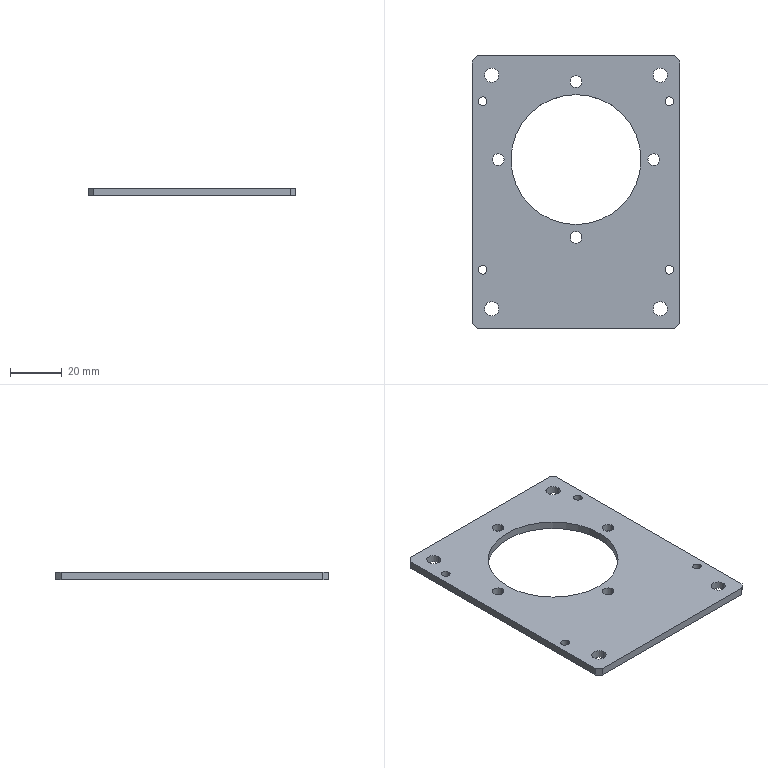Part | SolidWorks | features HoleWzd 2, Chamfer 1, Extrusion 1, ICE 1 | 1 solid | 36 faces | box 80 x 105 x 3 mm | volume 18683 mm3 | cylinder 26 | plane 10 | commonest cylinder face diameters 3.3 x8 4.5 x8 5.5 x8 50.1 x2
STEP:
#1=CARTESIAN_POINT('',(5.65,87.5,0.));
#2=VERTEX_POINT('',#1);
#3=CARTESIAN_POINT('',(2.35,87.5,0.));
#4=VERTEX_POINT('',#3);
#5=CARTESIAN_POINT('',(4.,87.5,0.));
#6=DIRECTION('',(0.,0.,-1.));
#7=DIRECTION('',(-1.,0.,0.));
#8=AXIS2_PLACEMENT_3D('',#5,#6,#7);
#9=CIRCLE('',#8,1.65);
#10=EDGE_CURVE('',#2,#4,#9,.T.);
#11=ORIENTED_EDGE('',*,*,#10,.T.);
#12=CARTESIAN_POINT('',(2.35,87.5,3.));
#13=VERTEX_POINT('',#12);
#14=CARTESIAN_POINT('',(2.35,87.5,3.));
#15=DIRECTION('',(0.,0.,1.));
#16=VECTOR('',#15,1000.);
#17=LINE('',#14,#16);
#18=EDGE_CURVE('',#4,#13,#17,.T.);
#19=ORIENTED_EDGE('',*,*,#18,.T.);
#20=CARTESIAN_POINT('',(5.65,87.5,3.));
#21=VERTEX_POINT('',#20);
#22=CARTESIAN_POINT('',(4.,87.5,3.));
#23=DIRECTION('',(0.,0.,1.));
#24=DIRECTION('',(1.,0.,0.));
#25=AXIS2_PLACEMENT_3D('',#22,#23,#24);
#26=CIRCLE('',#25,1.65);
#27=EDGE_CURVE('',#13,#21,#26,.T.);
#28=ORIENTED_EDGE('',*,*,#27,.T.);
#29=CARTESIAN_POINT('',(5.65,87.5,3.));
#30=DIRECTION('',(0.,0.,1.));
#31=VECTOR('',#30,1000.);
#32=LINE('',#29,#31);
#33=EDGE_CURVE('',#2,#21,#32,.T.);
#34=ORIENTED_EDGE('',*,*,#33,.F.);
#35=EDGE_LOOP('',(#11,#19,#28,#34));
#36=FACE_OUTER_BOUND('',#35,.T.);
#37=CARTESIAN_POINT('',(4.,87.5,3.));
#38=DIRECTION('',(0.,0.,1.));
#39=DIRECTION('',(1.,0.,0.));
#40=AXIS2_PLACEMENT_3D('',#37,#38,#39);
#41=CYLINDRICAL_SURFACE('',#40,1.65);
#42=ADVANCED_FACE('',(#36),#41,.F.);
#43=CARTESIAN_POINT('',(77.65,87.5,0.));
#44=VERTEX_POINT('',#43);
#45=CARTESIAN_POINT('',(74.35,87.5,0.));
#46=VERTEX_POINT('',#45);
#47=CARTESIAN_POINT('',(76.,87.5,0.));
#48=DIRECTION('',(0.,0.,-1.));
#49=DIRECTION('',(-1.,0.,0.));
#50=AXIS2_PLACEMENT_3D('',#47,#48,#49);
#51=CIRCLE('',#50,1.65);
#52=EDGE_CURVE('',#44,#46,#51,.T.);
#53=ORIENTED_EDGE('',*,*,#52,.T.);
#54=CARTESIAN_POINT('',(74.35,87.5,3.));
#55=VERTEX_POINT('',#54);
#56=CARTESIAN_POINT('',(74.35,87.5,3.));
#57=DIRECTION('',(0.,0.,1.));
#58=VECTOR('',#57,1000.);
#59=LINE('',#56,#58);
#60=EDGE_CURVE('',#46,#55,#59,.T.);
#61=ORIENTED_EDGE('',*,*,#60,.T.);
#62=CARTESIAN_POINT('',(77.65,87.5,3.));
#63=VERTEX_POINT('',#62);
#64=CARTESIAN_POINT('',(76.,87.5,3.));
#65=DIRECTION('',(0.,0.,1.));
#66=DIRECTION('',(1.,0.,0.));
#67=AXIS2_PLACEMENT_3D('',#64,#65,#66);
#68=CIRCLE('',#67,1.65);
#69=EDGE_CURVE('',#55,#63,#68,.T.);
#70=ORIENTED_EDGE('',*,*,#69,.T.);
#71=CARTESIAN_POINT('',(77.65,87.5,3.));
#72=DIRECTION('',(0.,0.,1.));
#73=VECTOR('',#72,1000.);
#74=LINE('',#71,#73);
#75=EDGE_CURVE('',#44,#63,#74,.T.);
#76=ORIENTED_EDGE('',*,*,#75,.F.);
#77=EDGE_LOOP('',(#53,#61,#70,#76));
#78=FACE_OUTER_BOUND('',#77,.T.);
#79=CARTESIAN_POINT('',(76.,87.5,3.));
#80=DIRECTION('',(0.,0.,1.));
#81=DIRECTION('',(1.,0.,0.));
#82=AXIS2_PLACEMENT_3D('',#79,#80,#81);
#83=CYLINDRICAL_SURFACE('',#82,1.65);
#84=ADVANCED_FACE('',(#78),#83,.F.);
#85=CARTESIAN_POINT('',(77.65,22.5,0.));
#86=VERTEX_POINT('',#85);
#87=CARTESIAN_POINT('',(74.35,22.5,0.));
#88=VERTEX_POINT('',#87);
#89=CARTESIAN_POINT('',(76.,22.5,0.));
#90=DIRECTION('',(0.,0.,-1.));
#91=DIRECTION('',(-1.,0.,0.));
#92=AXIS2_PLACEMENT_3D('',#89,#90,#91);
#93=CIRCLE('',#92,1.65);
#94=EDGE_CURVE('',#86,#88,#93,.T.);
#95=ORIENTED_EDGE('',*,*,#94,.T.);
#96=CARTESIAN_POINT('',(74.35,22.5,3.));
#97=VERTEX_POINT('',#96);
#98=CARTESIAN_POINT('',(74.35,22.5,3.));
#99=DIRECTION('',(0.,0.,1.));
#100=VECTOR('',#99,1000.);
#101=LINE('',#98,#100);
#102=EDGE_CURVE('',#88,#97,#101,.T.);
#103=ORIENTED_EDGE('',*,*,#102,.T.);
#104=CARTESIAN_POINT('',(77.65,22.5,3.));
#105=VERTEX_POINT('',#104);
#106=CARTESIAN_POINT('',(76.,22.5,3.));
#107=DIRECTION('',(0.,0.,1.));
#108=DIRECTION('',(1.,0.,0.));
#109=AXIS2_PLACEMENT_3D('',#106,#107,#108);
#110=CIRCLE('',#109,1.65);
#111=EDGE_CURVE('',#97,#105,#110,.T.);
#112=ORIENTED_EDGE('',*,*,#111,.T.);
#113=CARTESIAN_POINT('',(77.65,22.5,3.));
#114=DIRECTION('',(0.,0.,1.));
#115=VECTOR('',#114,1000.);
#116=LINE('',#113,#115);
#117=EDGE_CURVE('',#86,#105,#116,.T.);
#118=ORIENTED_EDGE('',*,*,#117,.F.);
#119=EDGE_LOOP('',(#95,#103,#112,#118));
#120=FACE_OUTER_BOUND('',#119,.T.);
#121=CARTESIAN_POINT('',(76.,22.5,3.));
#122=DIRECTION('',(0.,0.,1.));
#123=DIRECTION('',(1.,0.,0.));
#124=AXIS2_PLACEMENT_3D('',#121,#122,#123);
#125=CYLINDRICAL_SURFACE('',#124,1.65);
#126=ADVANCED_FACE('',(#120),#125,.F.);
#127=CARTESIAN_POINT('',(5.65,22.5,0.));
#128=VERTEX_POINT('',#127);
#129=CARTESIAN_POINT('',(2.35,22.5,0.));
#130=VERTEX_POINT('',#129);
#131=CARTESIAN_POINT('',(4.,22.5,0.));
#132=DIRECTION('',(0.,0.,-1.));
#133=DIRECTION('',(-1.,0.,0.));
#134=AXIS2_PLACEMENT_3D('',#131,#132,#133);
#135=CIRCLE('',#134,1.65);
#136=EDGE_CURVE('',#128,#130,#135,.T.);
#137=ORIENTED_EDGE('',*,*,#136,.T.);
#138=CARTESIAN_POINT('',(2.35,22.5,3.));
#139=VERTEX_POINT('',#138);
#140=CARTESIAN_POINT('',(2.35,22.5,3.));
#141=DIRECTION('',(0.,0.,1.));
#142=VECTOR('',#141,1000.);
#143=LINE('',#140,#142);
#144=EDGE_CURVE('',#130,#139,#143,.T.);
#145=ORIENTED_EDGE('',*,*,#144,.T.);
#146=CARTESIAN_POINT('',(5.65,22.5,3.));
#147=VERTEX_POINT('',#146);
#148=CARTESIAN_POINT('',(4.,22.5,3.));
#149=DIRECTION('',(0.,0.,1.));
#150=DIRECTION('',(1.,0.,0.));
#151=AXIS2_PLACEMENT_3D('',#148,#149,#150);
#152=CIRCLE('',#151,1.65);
#153=EDGE_CURVE('',#139,#147,#152,.T.);
#154=ORIENTED_EDGE('',*,*,#153,.T.);
#155=CARTESIAN_POINT('',(5.65,22.5,3.));
#156=DIRECTION('',(0.,0.,1.));
#157=VECTOR('',#156,1000.);
#158=LINE('',#155,#157);
#159=EDGE_CURVE('',#128,#147,#158,.T.);
#160=ORIENTED_EDGE('',*,*,#159,.F.);
#161=EDGE_LOOP('',(#137,#145,#154,#160));
#162=FACE_OUTER_BOUND('',#161,.T.);
#163=CARTESIAN_POINT('',(4.,22.5,3.));
#164=DIRECTION('',(0.,0.,1.));
#165=DIRECTION('',(1.,0.,0.));
#166=AXIS2_PLACEMENT_3D('',#163,#164,#165);
#167=CYLINDRICAL_SURFACE('',#166,1.65);
#168=ADVANCED_FACE('',(#162),#167,.F.);
#169=CARTESIAN_POINT('',(37.75,95.,0.));
#170=VERTEX_POINT('',#169);
#171=CARTESIAN_POINT('',(42.25,95.,0.));
#172=VERTEX_POINT('',#171);
#173=CARTESIAN_POINT('',(40.,95.,0.));
#174=DIRECTION('',(0.,0.,1.));
#175=DIRECTION('',(1.,0.,0.));
#176=AXIS2_PLACEMENT_3D('',#173,#174,#175);
#177=CIRCLE('',#176,2.25);
#178=EDGE_CURVE('',#170,#172,#177,.T.);
#179=ORIENTED_EDGE('',*,*,#178,.F.);
#180=CARTESIAN_POINT('',(37.75,95.,3.));
#181=VERTEX_POINT('',#180);
#182=CARTESIAN_POINT('',(37.75,95.,3.));
#183=DIRECTION('',(0.,0.,1.));
#184=VECTOR('',#183,1000.);
#185=LINE('',#182,#184);
#186=EDGE_CURVE('',#170,#181,#185,.T.);
#187=ORIENTED_EDGE('',*,*,#186,.T.);
#188=CARTESIAN_POINT('',(42.25,95.,3.));
#189=VERTEX_POINT('',#188);
#190=CARTESIAN_POINT('',(40.,95.,3.));
#191=DIRECTION('',(0.,0.,1.));
#192=DIRECTION('',(1.,0.,0.));
#193=AXIS2_PLACEMENT_3D('',#190,#191,#192);
#194=CIRCLE('',#193,2.25);
#195=EDGE_CURVE('',#181,#189,#194,.T.);
#196=ORIENTED_EDGE('',*,*,#195,.T.);
#197=CARTESIAN_POINT('',(42.25,95.,3.));
#198=DIRECTION('',(0.,0.,1.));
#199=VECTOR('',#198,1000.);
#200=LINE('',#197,#199);
#201=EDGE_CURVE('',#172,#189,#200,.T.);
#202=ORIENTED_EDGE('',*,*,#201,.F.);
#203=EDGE_LOOP('',(#179,#187,#196,#202));
#204=FACE_OUTER_BOUND('',#203,.T.);
#205=CARTESIAN_POINT('',(40.,95.,3.));
#206=DIRECTION('',(0.,0.,1.));
#207=DIRECTION('',(1.,0.,0.));
#208=AXIS2_PLACEMENT_3D('',#205,#206,#207);
#209=CYLINDRICAL_SURFACE('',#208,2.25);
#210=ADVANCED_FACE('',(#204),#209,.F.);
#211=CARTESIAN_POINT('',(7.75,65.,0.));
#212=VERTEX_POINT('',#211);
#213=CARTESIAN_POINT('',(12.25,65.,0.));
#214=VERTEX_POINT('',#213);
#215=CARTESIAN_POINT('',(10.,65.,0.));
#216=DIRECTION('',(0.,0.,1.));
#217=DIRECTION('',(1.,0.,0.));
#218=AXIS2_PLACEMENT_3D('',#215,#216,#217);
#219=CIRCLE('',#218,2.25);
#220=EDGE_CURVE('',#212,#214,#219,.T.);
#221=ORIENTED_EDGE('',*,*,#220,.F.);
#222=CARTESIAN_POINT('',(7.75,65.,3.));
#223=VERTEX_POINT('',#222);
#224=CARTESIAN_POINT('',(7.75,65.,3.));
#225=DIRECTION('',(0.,0.,1.));
#226=VECTOR('',#225,1000.);
#227=LINE('',#224,#226);
#228=EDGE_CURVE('',#212,#223,#227,.T.);
#229=ORIENTED_EDGE('',*,*,#228,.T.);
#230=CARTESIAN_POINT('',(12.25,65.,3.));
#231=VERTEX_POINT('',#230);
#232=CARTESIAN_POINT('',(10.,65.,3.));
#233=DIRECTION('',(0.,0.,1.));
#234=DIRECTION('',(1.,0.,0.));
#235=AXIS2_PLACEMENT_3D('',#232,#233,#234);
#236=CIRCLE('',#235,2.25);
#237=EDGE_CURVE('',#223,#231,#236,.T.);
#238=ORIENTED_EDGE('',*,*,#237,.T.);
#239=CARTESIAN_POINT('',(12.25,65.,3.));
#240=DIRECTION('',(0.,0.,1.));
#241=VECTOR('',#240,1000.);
#242=LINE('',#239,#241);
#243=EDGE_CURVE('',#214,#231,#242,.T.);
#244=ORIENTED_EDGE('',*,*,#243,.F.);
#245=EDGE_LOOP('',(#221,#229,#238,#244));
#246=FACE_OUTER_BOUND('',#245,.T.);
#247=CARTESIAN_POINT('',(10.,65.,3.));
#248=DIRECTION('',(0.,0.,1.));
#249=DIRECTION('',(1.,0.,0.));
#250=AXIS2_PLACEMENT_3D('',#247,#248,#249);
#251=CYLINDRICAL_SURFACE('',#250,2.25);
#252=ADVANCED_FACE('',(#246),#251,.F.);
#253=CARTESIAN_POINT('',(67.75,65.,0.));
#254=VERTEX_POINT('',#253);
#255=CARTESIAN_POINT('',(72.25,65.,0.));
#256=VERTEX_POINT('',#255);
#257=CARTESIAN_POINT('',(70.,65.,0.));
#258=DIRECTION('',(0.,0.,1.));
#259=DIRECTION('',(1.,0.,0.));
#260=AXIS2_PLACEMENT_3D('',#257,#258,#259);
#261=CIRCLE('',#260,2.25);
#262=EDGE_CURVE('',#254,#256,#261,.T.);
#263=ORIENTED_EDGE('',*,*,#262,.F.);
#264=CARTESIAN_POINT('',(67.75,65.,3.));
#265=VERTEX_POINT('',#264);
#266=CARTESIAN_POINT('',(67.75,65.,3.));
#267=DIRECTION('',(0.,0.,1.));
#268=VECTOR('',#267,1000.);
#269=LINE('',#266,#268);
#270=EDGE_CURVE('',#254,#265,#269,.T.);
#271=ORIENTED_EDGE('',*,*,#270,.T.);
#272=CARTESIAN_POINT('',(72.25,65.,3.));
#273=VERTEX_POINT('',#272);
#274=CARTESIAN_POINT('',(70.,65.,3.));
#275=DIRECTION('',(0.,0.,1.));
#276=DIRECTION('',(1.,0.,0.));
#277=AXIS2_PLACEMENT_3D('',#274,#275,#276);
#278=CIRCLE('',#277,2.25);
#279=EDGE_CURVE('',#265,#273,#278,.T.);
#280=ORIENTED_EDGE('',*,*,#279,.T.);
#281=CARTESIAN_POINT('',(72.25,65.,3.));
#282=DIRECTION('',(0.,0.,1.));
#283=VECTOR('',#282,1000.);
#284=LINE('',#281,#283);
#285=EDGE_CURVE('',#256,#273,#284,.T.);
#286=ORIENTED_EDGE('',*,*,#285,.F.);
#287=EDGE_LOOP('',(#263,#271,#280,#286));
#288=FACE_OUTER_BOUND('',#287,.T.);
#289=CARTESIAN_POINT('',(70.,65.,3.));
#290=DIRECTION('',(0.,0.,1.));
#291=DIRECTION('',(1.,0.,0.));
#292=AXIS2_PLACEMENT_3D('',#289,#290,#291);
#293=CYLINDRICAL_SURFACE('',#292,2.25);
#294=ADVANCED_FACE('',(#288),#293,.F.);
#295=CARTESIAN_POINT('',(37.75,35.,0.));
#296=VERTEX_POINT('',#295);
#297=CARTESIAN_POINT('',(42.25,35.,0.));
#298=VERTEX_POINT('',#297);
#299=CARTESIAN_POINT('',(40.,35.,0.));
#300=DIRECTION('',(0.,0.,1.));
#301=DIRECTION('',(1.,0.,0.));
#302=AXIS2_PLACEMENT_3D('',#299,#300,#301);
#303=CIRCLE('',#302,2.25);
#304=EDGE_CURVE('',#296,#298,#303,.T.);
#305=ORIENTED_EDGE('',*,*,#304,.F.);
#306=CARTESIAN_POINT('',(37.75,35.,3.));
#307=VERTEX_POINT('',#306);
#308=CARTESIAN_POINT('',(37.75,35.,3.));
#309=DIRECTION('',(0.,0.,1.));
#310=VECTOR('',#309,1000.);
#311=LINE('',#308,#310);
#312=EDGE_CURVE('',#296,#307,#311,.T.);
#313=ORIENTED_EDGE('',*,*,#312,.T.);
#314=CARTESIAN_POINT('',(42.25,35.,3.));
#315=VERTEX_POINT('',#314);
#316=CARTESIAN_POINT('',(40.,35.,3.));
#317=DIRECTION('',(0.,0.,1.));
#318=DIRECTION('',(1.,0.,0.));
#319=AXIS2_PLACEMENT_3D('',#316,#317,#318);
#320=CIRCLE('',#319,2.25);
#321=EDGE_CURVE('',#307,#315,#320,.T.);
#322=ORIENTED_EDGE('',*,*,#321,.T.);
#323=CARTESIAN_POINT('',(42.25,35.,3.));
#324=DIRECTION('',(0.,0.,1.));
#325=VECTOR('',#324,1000.);
#326=LINE('',#323,#325);
#327=EDGE_CURVE('',#298,#315,#326,.T.);
#328=ORIENTED_EDGE('',*,*,#327,.F.);
#329=EDGE_LOOP('',(#305,#313,#322,#328));
#330=FACE_OUTER_BOUND('',#329,.T.);
#331=CARTESIAN_POINT('',(40.,35.,3.));
#332=DIRECTION('',(0.,0.,1.));
#333=DIRECTION('',(1.,0.,0.));
#334=AXIS2_PLACEMENT_3D('',#331,#332,#333);
#335=CYLINDRICAL_SURFACE('',#334,2.25);
#336=ADVANCED_FACE('',(#330),#335,.F.);
#337=CARTESIAN_POINT('',(14.95,65.,0.));
#338=VERTEX_POINT('',#337);
#339=CARTESIAN_POINT('',(65.05,65.,0.));
#340=VERTEX_POINT('',#339);
#341=CARTESIAN_POINT('',(40.,65.,0.));
#342=DIRECTION('',(0.,0.,1.));
#343=DIRECTION('',(1.,0.,0.));
#344=AXIS2_PLACEMENT_3D('',#341,#342,#343);
#345=CIRCLE('',#344,25.05);
#346=EDGE_CURVE('',#338,#340,#345,.T.);
#347=ORIENTED_EDGE('',*,*,#346,.F.);
#348=CARTESIAN_POINT('',(14.95,65.,3.));
#349=VERTEX_POINT('',#348);
#350=CARTESIAN_POINT('',(14.95,65.,0.));
#351=DIRECTION('',(0.,0.,1.));
#352=VECTOR('',#351,1000.);
#353=LINE('',#350,#352);
#354=EDGE_CURVE('',#338,#349,#353,.T.);
#355=ORIENTED_EDGE('',*,*,#354,.T.);
#356=CARTESIAN_POINT('',(65.05,65.,3.));
#357=VERTEX_POINT('',#356);
#358=CARTESIAN_POINT('',(40.,65.,3.));
#359=DIRECTION('',(0.,0.,1.));
#360=DIRECTION('',(1.,0.,0.));
#361=AXIS2_PLACEMENT_3D('',#358,#359,#360);
#362=CIRCLE('',#361,25.05);
#363=EDGE_CURVE('',#349,#357,#362,.T.);
#364=ORIENTED_EDGE('',*,*,#363,.T.);
#365=CARTESIAN_POINT('',(65.05,65.,0.));
#366=DIRECTION('',(0.,0.,1.));
#367=VECTOR('',#366,1000.);
#368=LINE('',#365,#367);
#369=EDGE_CURVE('',#340,#357,#368,.T.);
#370=ORIENTED_EDGE('',*,*,#369,.F.);
#371=EDGE_LOOP('',(#347,#355,#364,#370));
#372=FACE_OUTER_BOUND('',#371,.T.);
#373=CARTESIAN_POINT('',(40.,65.,0.));
#374=DIRECTION('',(0.,0.,1.));
#375=DIRECTION('',(1.,0.,0.));
#376=AXIS2_PLACEMENT_3D('',#373,#374,#375);
#377=CYLINDRICAL_SURFACE('',#376,25.05);
#378=ADVANCED_FACE('',(#372),#377,.F.);
#379=CARTESIAN_POINT('',(4.75,7.5,0.));
#380=VERTEX_POINT('',#379);
#381=CARTESIAN_POINT('',(10.25,7.5,0.));
#382=VERTEX_POINT('',#381);
#383=CARTESIAN_POINT('',(7.5,7.5,0.));
#384=DIRECTION('',(0.,0.,1.));
#385=DIRECTION('',(1.,0.,0.));
#386=AXIS2_PLACEMENT_3D('',#383,#384,#385);
#387=CIRCLE('',#386,2.75);
#388=EDGE_CURVE('',#380,#382,#387,.T.);
#389=ORIENTED_EDGE('',*,*,#388,.F.);
#390=CARTESIAN_POINT('',(4.75,7.5,3.));
#391=VERTEX_POINT('',#390);
#392=CARTESIAN_POINT('',(4.75,7.5,0.));
#393=DIRECTION('',(0.,0.,1.));
#394=VECTOR('',#393,1000.);
#395=LINE('',#392,#394);
#396=EDGE_CURVE('',#380,#391,#395,.T.);
#397=ORIENTED_EDGE('',*,*,#396,.T.);
#398=CARTESIAN_POINT('',(10.25,7.5,3.));
#399=VERTEX_POINT('',#398);
#400=CARTESIAN_POINT('',(7.5,7.5,3.));
#401=DIRECTION('',(0.,0.,1.));
#402=DIRECTION('',(1.,0.,0.));
#403=AXIS2_PLACEMENT_3D('',#400,#401,#402);
#404=CIRCLE('',#403,2.75);
#405=EDGE_CURVE('',#391,#399,#404,.T.);
#406=ORIENTED_EDGE('',*,*,#405,.T.);
#407=CARTESIAN_POINT('',(10.25,7.5,0.));
#408=DIRECTION('',(0.,0.,1.));
#409=VECTOR('',#408,1000.);
#410=LINE('',#407,#409);
#411=EDGE_CURVE('',#382,#399,#410,.T.);
#412=ORIENTED_EDGE('',*,*,#411,.F.);
#413=EDGE_LOOP('',(#389,#397,#406,#412));
#414=FACE_OUTER_BOUND('',#413,.T.);
#415=CARTESIAN_POINT('',(7.5,7.5,0.));
#416=DIRECTION('',(0.,0.,1.));
#417=DIRECTION('',(1.,0.,0.));
#418=AXIS2_PLACEMENT_3D('',#415,#416,#417);
#419=CYLINDRICAL_SURFACE('',#418,2.75);
#420=ADVANCED_FACE('',(#414),#419,.F.);
#421=CARTESIAN_POINT('',(69.75,7.5,0.));
#422=VERTEX_POINT('',#421);
#423=CARTESIAN_POINT('',(75.25,7.5,0.));
#424=VERTEX_POINT('',#423);
#425=CARTESIAN_POINT('',(72.5,7.5,0.));
#426=DIRECTION('',(0.,0.,1.));
#427=DIRECTION('',(1.,0.,0.));
#428=AXIS2_PLACEMENT_3D('',#425,#426,#427);
#429=CIRCLE('',#428,2.75);
#430=EDGE_CURVE('',#422,#424,#429,.T.);
#431=ORIENTED_EDGE('',*,*,#430,.F.);
#432=CARTESIAN_POINT('',(69.75,7.5,3.));
#433=VERTEX_POINT('',#432);
#434=CARTESIAN_POINT('',(69.75,7.5,0.));
#435=DIRECTION('',(0.,0.,1.));
#436=VECTOR('',#435,1000.);
#437=LINE('',#434,#436);
#438=EDGE_CURVE('',#422,#433,#437,.T.);
#439=ORIENTED_EDGE('',*,*,#438,.T.);
#440=CARTESIAN_POINT('',(75.25,7.5,3.));
#441=VERTEX_POINT('',#440);
#442=CARTESIAN_POINT('',(72.5,7.5,3.));
#443=DIRECTION('',(0.,0.,1.));
#444=DIRECTION('',(1.,0.,0.));
#445=AXIS2_PLACEMENT_3D('',#442,#443,#444);
#446=CIRCLE('',#445,2.75);
#447=EDGE_CURVE('',#433,#441,#446,.T.);
#448=ORIENTED_EDGE('',*,*,#447,.T.);
#449=CARTESIAN_POINT('',(75.25,7.5,0.));
#450=DIRECTION('',(0.,0.,1.));
#451=VECTOR('',#450,1000.);
#452=LINE('',#449,#451);
#453=EDGE_CURVE('',#424,#441,#452,.T.);
#454=ORIENTED_EDGE('',*,*,#453,.F.);
#455=EDGE_LOOP('',(#431,#439,#448,#454));
#456=FACE_OUTER_BOUND('',#455,.T.);
#457=CARTESIAN_POINT('',(72.5,7.5,0.));
#458=DIRECTION('',(0.,0.,1.));
#459=DIRECTION('',(1.,0.,0.));
#460=AXIS2_PLACEMENT_3D('',#457,#458,#459);
#461=CYLINDRICAL_SURFACE('',#460,2.75);
#462=ADVANCED_FACE('',(#456),#461,.F.);
#463=CARTESIAN_POINT('',(69.75,97.5,0.));
#464=VERTEX_POINT('',#463);
#465=CARTESIAN_POINT('',(75.25,97.5,0.));
#466=VERTEX_POINT('',#465);
#467=CARTESIAN_POINT('',(72.5,97.5,0.));
#468=DIRECTION('',(0.,0.,1.));
#469=DIRECTION('',(1.,0.,0.));
#470=AXIS2_PLACEMENT_3D('',#467,#468,#469);
#471=CIRCLE('',#470,2.75);
#472=EDGE_CURVE('',#464,#466,#471,.T.);
#473=ORIENTED_EDGE('',*,*,#472,.F.);
#474=CARTESIAN_POINT('',(69.75,97.5,3.));
#475=VERTEX_POINT('',#474);
#476=CARTESIAN_POINT('',(69.75,97.5,0.));
#477=DIRECTION('',(0.,0.,1.));
#478=VECTOR('',#477,1000.);
#479=LINE('',#476,#478);
#480=EDGE_CURVE('',#464,#475,#479,.T.);
#481=ORIENTED_EDGE('',*,*,#480,.T.);
#482=CARTESIAN_POINT('',(75.25,97.5,3.));
#483=VERTEX_POINT('',#482);
#484=CARTESIAN_POINT('',(72.5,97.5,3.));
#485=DIRECTION('',(0.,0.,1.));
#486=DIRECTION('',(1.,0.,0.));
#487=AXIS2_PLACEMENT_3D('',#484,#485,#486);
#488=CIRCLE('',#487,2.75);
#489=EDGE_CURVE('',#475,#483,#488,.T.);
#490=ORIENTED_EDGE('',*,*,#489,.T.);
#491=CARTESIAN_POINT('',(75.25,97.5,0.));
#492=DIRECTION('',(0.,0.,1.));
#493=VECTOR('',#492,1000.);
#494=LINE('',#491,#493);
#495=EDGE_CURVE('',#466,#483,#494,.T.);
#496=ORIENTED_EDGE('',*,*,#495,.F.);
#497=EDGE_LOOP('',(#473,#481,#490,#496));
#498=FACE_OUTER_BOUND('',#497,.T.);
#499=CARTESIAN_POINT('',(72.5,97.5,0.));
#500=DIRECTION('',(0.,0.,1.));
#501=DIRECTION('',(1.,0.,0.));
#502=AXIS2_PLACEMENT_3D('',#499,#500,#501);
#503=CYLINDRICAL_SURFACE('',#502,2.75);
#504=ADVANCED_FACE('',(#498),#503,.F.);
#505=CARTESIAN_POINT('',(4.75,97.5,0.));
#506=VERTEX_POINT('',#505);
#507=CARTESIAN_POINT('',(10.25,97.5,0.));
#508=VERTEX_POINT('',#507);
#509=CARTESIAN_POINT('',(7.5,97.5,0.));
#510=DIRECTION('',(0.,0.,1.));
#511=DIRECTION('',(1.,0.,0.));
#512=AXIS2_PLACEMENT_3D('',#509,#510,#511);
#513=CIRCLE('',#512,2.75);
#514=EDGE_CURVE('',#506,#508,#513,.T.);
#515=ORIENTED_EDGE('',*,*,#514,.F.);
#516=CARTESIAN_POINT('',(4.75,97.5,3.));
#517=VERTEX_POINT('',#516);
#518=CARTESIAN_POINT('',(4.75,97.5,0.));
#519=DIRECTION('',(0.,0.,1.));
#520=VECTOR('',#519,1000.);
#521=LINE('',#518,#520);
#522=EDGE_CURVE('',#506,#517,#521,.T.);
#523=ORIENTED_EDGE('',*,*,#522,.T.);
#524=CARTESIAN_POINT('',(10.25,97.5,3.));
#525=VERTEX_POINT('',#524);
#526=CARTESIAN_POINT('',(7.5,97.5,3.));
#527=DIRECTION('',(0.,0.,1.));
#528=DIRECTION('',(1.,0.,0.));
#529=AXIS2_PLACEMENT_3D('',#526,#527,#528);
#530=CIRCLE('',#529,2.75);
#531=EDGE_CURVE('',#517,#525,#530,.T.);
#532=ORIENTED_EDGE('',*,*,#531,.T.);
#533=CARTESIAN_POINT('',(10.25,97.5,0.));
#534=DIRECTION('',(0.,0.,1.));
#535=VECTOR('',#534,1000.);
#536=LINE('',#533,#535);
#537=EDGE_CURVE('',#508,#525,#536,.T.);
#538=ORIENTED_EDGE('',*,*,#537,.F.);
#539=EDGE_LOOP('',(#515,#523,#532,#538));
#540=FACE_OUTER_BOUND('',#539,.T.);
#541=CARTESIAN_POINT('',(7.5,97.5,0.));
#542=DIRECTION('',(0.,0.,1.));
#543=DIRECTION('',(1.,0.,0.));
#544=AXIS2_PLACEMENT_3D('',#541,#542,#543);
#545=CYLINDRICAL_SURFACE('',#544,2.75);
#546=ADVANCED_FACE('',(#540),#545,.F.);
#547=CARTESIAN_POINT('',(0.,103.,0.));
#548=VERTEX_POINT('',#547);
#549=CARTESIAN_POINT('',(0.,2.,0.));
#550=VERTEX_POINT('',#549);
#551=CARTESIAN_POINT('',(0.,0.,0.));
#552=DIRECTION('',(0.,-1.,0.));
#553=VECTOR('',#552,1000.);
#554=LINE('',#551,#553);
#555=EDGE_CURVE('',#548,#550,#554,.T.);
#556=ORIENTED_EDGE('',*,*,#555,.T.);
#557=CARTESIAN_POINT('',(0.,2.,3.));
#558=VERTEX_POINT('',#557);
#559=CARTESIAN_POINT('',(0.,2.,3.));
#560=DIRECTION('',(0.,0.,1.));
#561=VECTOR('',#560,1000.);
#562=LINE('',#559,#561);
#563=EDGE_CURVE('',#550,#558,#562,.T.);
#564=ORIENTED_EDGE('',*,*,#563,.T.);
#565=CARTESIAN_POINT('',(0.,103.,3.));
#566=VERTEX_POINT('',#565);
#567=CARTESIAN_POINT('',(0.,0.,3.));
#568=DIRECTION('',(0.,-1.,0.));
#569=VECTOR('',#568,1000.);
#570=LINE('',#567,#569);
#571=EDGE_CURVE('',#566,#558,#570,.T.);
#572=ORIENTED_EDGE('',*,*,#571,.F.);
#573=CARTESIAN_POINT('',(0.,103.,3.));
#574=DIRECTION('',(0.,0.,-1.));
#575=VECTOR('',#574,1000.);
#576=LINE('',#573,#575);
#577=EDGE_CURVE('',#566,#548,#576,.T.);
#578=ORIENTED_EDGE('',*,*,#577,.T.);
#579=EDGE_LOOP('',(#556,#564,#572,#578));
#580=FACE_OUTER_BOUND('',#579,.T.);
#581=CARTESIAN_POINT('',(0.,0.,3.));
#582=DIRECTION('',(1.,0.,0.));
#583=DIRECTION('',(0.,0.,-1.));
#584=AXIS2_PLACEMENT_3D('',#581,#582,#583);
#585=PLANE('',#584);
#586=ADVANCED_FACE('',(#580),#585,.F.);
#587=CARTESIAN_POINT('',(2.,0.,0.));
#588=VERTEX_POINT('',#587);
#589=CARTESIAN_POINT('',(78.,0.,0.));
#590=VERTEX_POINT('',#589);
#591=CARTESIAN_POINT('',(0.,0.,0.));
#592=DIRECTION('',(1.,0.,0.));
#593=VECTOR('',#592,1000.);
#594=LINE('',#591,#593);
#595=EDGE_CURVE('',#588,#590,#594,.T.);
#596=ORIENTED_EDGE('',*,*,#595,.T.);
#597=CARTESIAN_POINT('',(78.,0.,3.));
#598=VERTEX_POINT('',#597);
#599=CARTESIAN_POINT('',(78.,0.,3.));
#600=DIRECTION('',(0.,0.,1.));
#601=VECTOR('',#600,1000.);
#602=LINE('',#599,#601);
#603=EDGE_CURVE('',#590,#598,#602,.T.);
#604=ORIENTED_EDGE('',*,*,#603,.T.);
#605=CARTESIAN_POINT('',(2.,0.,3.));
#606=VERTEX_POINT('',#605);
#607=CARTESIAN_POINT('',(0.,0.,3.));
#608=DIRECTION('',(1.,0.,0.));
#609=VECTOR('',#608,1000.);
#610=LINE('',#607,#609);
#611=EDGE_CURVE('',#606,#598,#610,.T.);
#612=ORIENTED_EDGE('',*,*,#611,.F.);
#613=CARTESIAN_POINT('',(2.,0.,3.));
#614=DIRECTION('',(0.,0.,-1.));
#615=VECTOR('',#614,1000.);
#616=LINE('',#613,#615);
#617=EDGE_CURVE('',#606,#588,#616,.T.);
#618=ORIENTED_EDGE('',*,*,#617,.T.);
#619=EDGE_LOOP('',(#596,#604,#612,#618));
#620=FACE_OUTER_BOUND('',#619,.T.);
#621=CARTESIAN_POINT('',(0.,0.,3.));
#622=DIRECTION('',(0.,1.,0.));
#623=DIRECTION('',(0.,0.,1.));
#624=AXIS2_PLACEMENT_3D('',#621,#622,#623);
#625=PLANE('',#624);
#626=ADVANCED_FACE('',(#620),#625,.F.);
#627=CARTESIAN_POINT('',(80.,2.,3.));
#628=VERTEX_POINT('',#627);
#629=CARTESIAN_POINT('',(80.,103.,3.));
#630=VERTEX_POINT('',#629);
#631=CARTESIAN_POINT('',(80.,0.,3.));
#632=DIRECTION('',(0.,1.,0.));
#633=VECTOR('',#632,1000.);
#634=LINE('',#631,#633);
#635=EDGE_CURVE('',#628,#630,#634,.T.);
#636=ORIENTED_EDGE('',*,*,#635,.F.);
#637=CARTESIAN_POINT('',(80.,2.,0.));
#638=VERTEX_POINT('',#637);
#639=CARTESIAN_POINT('',(80.,2.,3.));
#640=DIRECTION('',(0.,0.,-1.));
#641=VECTOR('',#640,1000.);
#642=LINE('',#639,#641);
#643=EDGE_CURVE('',#628,#638,#642,.T.);
#644=ORIENTED_EDGE('',*,*,#643,.T.);
#645=CARTESIAN_POINT('',(80.,103.,0.));
#646=VERTEX_POINT('',#645);
#647=CARTESIAN_POINT('',(80.,0.,0.));
#648=DIRECTION('',(0.,1.,0.));
#649=VECTOR('',#648,1000.);
#650=LINE('',#647,#649);
#651=EDGE_CURVE('',#638,#646,#650,.T.);
#652=ORIENTED_EDGE('',*,*,#651,.T.);
#653=CARTESIAN_POINT('',(80.,103.,3.));
#654=DIRECTION('',(0.,0.,1.));
#655=VECTOR('',#654,1000.);
#656=LINE('',#653,#655);
#657=EDGE_CURVE('',#646,#630,#656,.T.);
#658=ORIENTED_EDGE('',*,*,#657,.T.);
#659=EDGE_LOOP('',(#636,#644,#652,#658));
#660=FACE_OUTER_BOUND('',#659,.T.);
#661=CARTESIAN_POINT('',(80.,0.,3.));
#662=DIRECTION('',(-1.,0.,0.));
#663=DIRECTION('',(0.,0.,1.));
#664=AXIS2_PLACEMENT_3D('',#661,#662,#663);
#665=PLANE('',#664);
#666=ADVANCED_FACE('',(#660),#665,.F.);
#667=CARTESIAN_POINT('',(78.,105.,3.));
#668=VERTEX_POINT('',#667);
#669=CARTESIAN_POINT('',(2.,105.,3.));
#670=VERTEX_POINT('',#669);
#671=CARTESIAN_POINT('',(0.,105.,3.));
#672=DIRECTION('',(-1.,0.,0.));
#673=VECTOR('',#672,1000.);
#674=LINE('',#671,#673);
#675=EDGE_CURVE('',#668,#670,#674,.T.);
#676=ORIENTED_EDGE('',*,*,#675,.F.);
#677=CARTESIAN_POINT('',(78.,105.,0.));
#678=VERTEX_POINT('',#677);
#679=CARTESIAN_POINT('',(78.,105.,3.));
#680=DIRECTION('',(0.,0.,-1.));
#681=VECTOR('',#680,1000.);
#682=LINE('',#679,#681);
#683=EDGE_CURVE('',#668,#678,#682,.T.);
#684=ORIENTED_EDGE('',*,*,#683,.T.);
#685=CARTESIAN_POINT('',(2.,105.,0.));
#686=VERTEX_POINT('',#685);
#687=CARTESIAN_POINT('',(0.,105.,0.));
#688=DIRECTION('',(-1.,0.,0.));
#689=VECTOR('',#688,1000.);
#690=LINE('',#687,#689);
#691=EDGE_CURVE('',#678,#686,#690,.T.);
#692=ORIENTED_EDGE('',*,*,#691,.T.);
#693=CARTESIAN_POINT('',(2.,105.,3.));
#694=DIRECTION('',(0.,0.,1.));
#695=VECTOR('',#694,1000.);
#696=LINE('',#693,#695);
#697=EDGE_CURVE('',#686,#670,#696,.T.);
#698=ORIENTED_EDGE('',*,*,#697,.T.);
#699=EDGE_LOOP('',(#676,#684,#692,#698));
#700=FACE_OUTER_BOUND('',#699,.T.);
#701=CARTESIAN_POINT('',(0.,105.,3.));
#702=DIRECTION('',(0.,-1.,0.));
#703=DIRECTION('',(0.,0.,-1.));
#704=AXIS2_PLACEMENT_3D('',#701,#702,#703);
#705=PLANE('',#704);
#706=ADVANCED_FACE('',(#700),#705,.F.);
#707=CARTESIAN_POINT('',(4.,87.5,3.));
#708=DIRECTION('',(0.,0.,1.));
#709=DIRECTION('',(1.,0.,0.));
#710=AXIS2_PLACEMENT_3D('',#707,#708,#709);
#711=CIRCLE('',#710,1.65);
#712=EDGE_CURVE('',#21,#13,#711,.T.);
#713=ORIENTED_EDGE('',*,*,#712,.F.);
#714=ORIENTED_EDGE('',*,*,#27,.F.);
#715=EDGE_LOOP('',(#713,#714));
#716=FACE_BOUND('',#715,.T.);
#717=CARTESIAN_POINT('',(76.,87.5,3.));
#718=DIRECTION('',(0.,0.,1.));
#719=DIRECTION('',(1.,0.,0.));
#720=AXIS2_PLACEMENT_3D('',#717,#718,#719);
#721=CIRCLE('',#720,1.65);
#722=EDGE_CURVE('',#63,#55,#721,.T.);
#723=ORIENTED_EDGE('',*,*,#722,.F.);
#724=ORIENTED_EDGE('',*,*,#69,.F.);
#725=EDGE_LOOP('',(#723,#724));
#726=FACE_BOUND('',#725,.T.);
#727=CARTESIAN_POINT('',(76.,22.5,3.));
#728=DIRECTION('',(0.,0.,1.));
#729=DIRECTION('',(1.,0.,0.));
#730=AXIS2_PLACEMENT_3D('',#727,#728,#729);
#731=CIRCLE('',#730,1.65);
#732=EDGE_CURVE('',#105,#97,#731,.T.);
#733=ORIENTED_EDGE('',*,*,#732,.F.);
#734=ORIENTED_EDGE('',*,*,#111,.F.);
#735=EDGE_LOOP('',(#733,#734));
#736=FACE_BOUND('',#735,.T.);
#737=CARTESIAN_POINT('',(4.,22.5,3.));
#738=DIRECTION('',(0.,0.,1.));
#739=DIRECTION('',(1.,0.,0.));
#740=AXIS2_PLACEMENT_3D('',#737,#738,#739);
#741=CIRCLE('',#740,1.65);
#742=EDGE_CURVE('',#147,#139,#741,.T.);
#743=ORIENTED_EDGE('',*,*,#742,.F.);
#744=ORIENTED_EDGE('',*,*,#153,.F.);
#745=EDGE_LOOP('',(#743,#744));
#746=FACE_BOUND('',#745,.T.);
#747=CARTESIAN_POINT('',(40.,95.,3.));
#748=DIRECTION('',(0.,0.,1.));
#749=DIRECTION('',(1.,0.,0.));
#750=AXIS2_PLACEMENT_3D('',#747,#748,#749);
#751=CIRCLE('',#750,2.25);
#752=EDGE_CURVE('',#189,#181,#751,.T.);
#753=ORIENTED_EDGE('',*,*,#752,.F.);
#754=ORIENTED_EDGE('',*,*,#195,.F.);
#755=EDGE_LOOP('',(#753,#754));
#756=FACE_BOUND('',#755,.T.);
#757=CARTESIAN_POINT('',(10.,65.,3.));
#758=DIRECTION('',(0.,0.,1.));
#759=DIRECTION('',(1.,0.,0.));
#760=AXIS2_PLACEMENT_3D('',#757,#758,#759);
#761=CIRCLE('',#760,2.25);
#762=EDGE_CURVE('',#231,#223,#761,.T.);
#763=ORIENTED_EDGE('',*,*,#762,.F.);
#764=ORIENTED_EDGE('',*,*,#237,.F.);
#765=EDGE_LOOP('',(#763,#764));
#766=FACE_BOUND('',#765,.T.);
#767=CARTESIAN_POINT('',(70.,65.,3.));
#768=DIRECTION('',(0.,0.,1.));
#769=DIRECTION('',(1.,0.,0.));
#770=AXIS2_PLACEMENT_3D('',#767,#768,#769);
#771=CIRCLE('',#770,2.25);
#772=EDGE_CURVE('',#273,#265,#771,.T.);
#773=ORIENTED_EDGE('',*,*,#772,.F.);
#774=ORIENTED_EDGE('',*,*,#279,.F.);
#775=EDGE_LOOP('',(#773,#774));
#776=FACE_BOUND('',#775,.T.);
#777=CARTESIAN_POINT('',(40.,35.,3.));
#778=DIRECTION('',(0.,0.,1.));
#779=DIRECTION('',(1.,0.,0.));
#780=AXIS2_PLACEMENT_3D('',#777,#778,#779);
#781=CIRCLE('',#780,2.25);
#782=EDGE_CURVE('',#315,#307,#781,.T.);
#783=ORIENTED_EDGE('',*,*,#782,.F.);
#784=ORIENTED_EDGE('',*,*,#321,.F.);
#785=EDGE_LOOP('',(#783,#784));
#786=FACE_BOUND('',#785,.T.);
#787=CARTESIAN_POINT('',(40.,65.,3.));
#788=DIRECTION('',(0.,0.,1.));
#789=DIRECTION('',(1.,0.,0.));
#790=AXIS2_PLACEMENT_3D('',#787,#788,#789);
#791=CIRCLE('',#790,25.05);
#792=EDGE_CURVE('',#357,#349,#791,.T.);
#793=ORIENTED_EDGE('',*,*,#792,.F.);
#794=ORIENTED_EDGE('',*,*,#363,.F.);
#795=EDGE_LOOP('',(#793,#794));
#796=FACE_BOUND('',#795,.T.);
#797=CARTESIAN_POINT('',(7.5,7.5,3.));
#798=DIRECTION('',(0.,0.,1.));
#799=DIRECTION('',(1.,0.,0.));
#800=AXIS2_PLACEMENT_3D('',#797,#798,#799);
#801=CIRCLE('',#800,2.75);
#802=EDGE_CURVE('',#399,#391,#801,.T.);
#803=ORIENTED_EDGE('',*,*,#802,.F.);
#804=ORIENTED_EDGE('',*,*,#405,.F.);
#805=EDGE_LOOP('',(#803,#804));
#806=FACE_BOUND('',#805,.T.);
#807=CARTESIAN_POINT('',(72.5,7.5,3.));
#808=DIRECTION('',(0.,0.,1.));
#809=DIRECTION('',(1.,0.,0.));
#810=AXIS2_PLACEMENT_3D('',#807,#808,#809);
#811=CIRCLE('',#810,2.75);
#812=EDGE_CURVE('',#441,#433,#811,.T.);
#813=ORIENTED_EDGE('',*,*,#812,.F.);
#814=ORIENTED_EDGE('',*,*,#447,.F.);
#815=EDGE_LOOP('',(#813,#814));
#816=FACE_BOUND('',#815,.T.);
#817=CARTESIAN_POINT('',(72.5,97.5,3.));
#818=DIRECTION('',(0.,0.,1.));
#819=DIRECTION('',(1.,0.,0.));
#820=AXIS2_PLACEMENT_3D('',#817,#818,#819);
#821=CIRCLE('',#820,2.75);
#822=EDGE_CURVE('',#483,#475,#821,.T.);
#823=ORIENTED_EDGE('',*,*,#822,.F.);
#824=ORIENTED_EDGE('',*,*,#489,.F.);
#825=EDGE_LOOP('',(#823,#824));
#826=FACE_BOUND('',#825,.T.);
#827=CARTESIAN_POINT('',(7.5,97.5,3.));
#828=DIRECTION('',(0.,0.,1.));
#829=DIRECTION('',(1.,0.,0.));
#830=AXIS2_PLACEMENT_3D('',#827,#828,#829);
#831=CIRCLE('',#830,2.75);
#832=EDGE_CURVE('',#525,#517,#831,.T.);
#833=ORIENTED_EDGE('',*,*,#832,.F.);
#834=ORIENTED_EDGE('',*,*,#531,.F.);
#835=EDGE_LOOP('',(#833,#834));
#836=FACE_BOUND('',#835,.T.);
#837=ORIENTED_EDGE('',*,*,#611,.T.);
#838=CARTESIAN_POINT('',(80.,2.,3.));
#839=DIRECTION('',(0.7071,0.7071,0.));
#840=VECTOR('',#839,1000.);
#841=LINE('',#838,#840);
#842=EDGE_CURVE('',#598,#628,#841,.T.);
#843=ORIENTED_EDGE('',*,*,#842,.T.);
#844=ORIENTED_EDGE('',*,*,#635,.T.);
#845=CARTESIAN_POINT('',(78.,105.,3.));
#846=DIRECTION('',(-0.7071,0.7071,0.));
#847=VECTOR('',#846,1000.);
#848=LINE('',#845,#847);
#849=EDGE_CURVE('',#630,#668,#848,.T.);
#850=ORIENTED_EDGE('',*,*,#849,.T.);
#851=ORIENTED_EDGE('',*,*,#675,.T.);
#852=CARTESIAN_POINT('',(0.,103.,3.));
#853=DIRECTION('',(-0.7071,-0.7071,0.));
#854=VECTOR('',#853,1000.);
#855=LINE('',#852,#854);
#856=EDGE_CURVE('',#670,#566,#855,.T.);
#857=ORIENTED_EDGE('',*,*,#856,.T.);
#858=ORIENTED_EDGE('',*,*,#571,.T.);
#859=CARTESIAN_POINT('',(2.,0.,3.));
#860=DIRECTION('',(0.7071,-0.7071,0.));
#861=VECTOR('',#860,1000.);
#862=LINE('',#859,#861);
#863=EDGE_CURVE('',#558,#606,#862,.T.);
#864=ORIENTED_EDGE('',*,*,#863,.T.);
#865=EDGE_LOOP('',(#837,#843,#844,#850,#851,#857,#858,#864));
#866=FACE_OUTER_BOUND('',#865,.T.);
#867=CARTESIAN_POINT('',(0.,105.,3.));
#868=DIRECTION('',(0.,0.,-1.));
#869=DIRECTION('',(-1.,0.,0.));
#870=AXIS2_PLACEMENT_3D('',#867,#868,#869);
#871=PLANE('',#870);
#872=ADVANCED_FACE('',(#716,#726,#736,#746,#756,#766,#776,#786,#796,#806,#816,#826,#836,#866),#871,.F.);
#873=ORIENTED_EDGE('',*,*,#10,.F.);
#874=CARTESIAN_POINT('',(4.,87.5,0.));
#875=DIRECTION('',(0.,0.,-1.));
#876=DIRECTION('',(-1.,0.,0.));
#877=AXIS2_PLACEMENT_3D('',#874,#875,#876);
#878=CIRCLE('',#877,1.65);
#879=EDGE_CURVE('',#4,#2,#878,.T.);
#880=ORIENTED_EDGE('',*,*,#879,.F.);
#881=EDGE_LOOP('',(#873,#880));
#882=FACE_BOUND('',#881,.T.);
#883=ORIENTED_EDGE('',*,*,#52,.F.);
#884=CARTESIAN_POINT('',(76.,87.5,0.));
#885=DIRECTION('',(0.,0.,-1.));
#886=DIRECTION('',(-1.,0.,0.));
#887=AXIS2_PLACEMENT_3D('',#884,#885,#886);
#888=CIRCLE('',#887,1.65);
#889=EDGE_CURVE('',#46,#44,#888,.T.);
#890=ORIENTED_EDGE('',*,*,#889,.F.);
#891=EDGE_LOOP('',(#883,#890));
#892=FACE_BOUND('',#891,.T.);
#893=ORIENTED_EDGE('',*,*,#94,.F.);
#894=CARTESIAN_POINT('',(76.,22.5,0.));
#895=DIRECTION('',(0.,0.,-1.));
#896=DIRECTION('',(-1.,0.,0.));
#897=AXIS2_PLACEMENT_3D('',#894,#895,#896);
#898=CIRCLE('',#897,1.65);
#899=EDGE_CURVE('',#88,#86,#898,.T.);
#900=ORIENTED_EDGE('',*,*,#899,.F.);
#901=EDGE_LOOP('',(#893,#900));
#902=FACE_BOUND('',#901,.T.);
#903=ORIENTED_EDGE('',*,*,#136,.F.);
#904=CARTESIAN_POINT('',(4.,22.5,0.));
#905=DIRECTION('',(0.,0.,-1.));
#906=DIRECTION('',(-1.,0.,0.));
#907=AXIS2_PLACEMENT_3D('',#904,#905,#906);
#908=CIRCLE('',#907,1.65);
#909=EDGE_CURVE('',#130,#128,#908,.T.);
#910=ORIENTED_EDGE('',*,*,#909,.F.);
#911=EDGE_LOOP('',(#903,#910));
#912=FACE_BOUND('',#911,.T.);
#913=CARTESIAN_POINT('',(40.,95.,0.));
#914=DIRECTION('',(0.,0.,1.));
#915=DIRECTION('',(1.,0.,0.));
#916=AXIS2_PLACEMENT_3D('',#913,#914,#915);
#917=CIRCLE('',#916,2.25);
#918=EDGE_CURVE('',#172,#170,#917,.T.);
#919=ORIENTED_EDGE('',*,*,#918,.T.);
#920=ORIENTED_EDGE('',*,*,#178,.T.);
#921=EDGE_LOOP('',(#919,#920));
#922=FACE_BOUND('',#921,.T.);
#923=CARTESIAN_POINT('',(10.,65.,0.));
#924=DIRECTION('',(0.,0.,1.));
#925=DIRECTION('',(1.,0.,0.));
#926=AXIS2_PLACEMENT_3D('',#923,#924,#925);
#927=CIRCLE('',#926,2.25);
#928=EDGE_CURVE('',#214,#212,#927,.T.);
#929=ORIENTED_EDGE('',*,*,#928,.T.);
#930=ORIENTED_EDGE('',*,*,#220,.T.);
#931=EDGE_LOOP('',(#929,#930));
#932=FACE_BOUND('',#931,.T.);
#933=CARTESIAN_POINT('',(70.,65.,0.));
#934=DIRECTION('',(0.,0.,1.));
#935=DIRECTION('',(1.,0.,0.));
#936=AXIS2_PLACEMENT_3D('',#933,#934,#935);
#937=CIRCLE('',#936,2.25);
#938=EDGE_CURVE('',#256,#254,#937,.T.);
#939=ORIENTED_EDGE('',*,*,#938,.T.);
#940=ORIENTED_EDGE('',*,*,#262,.T.);
#941=EDGE_LOOP('',(#939,#940));
#942=FACE_BOUND('',#941,.T.);
#943=CARTESIAN_POINT('',(40.,35.,0.));
#944=DIRECTION('',(0.,0.,1.));
#945=DIRECTION('',(1.,0.,0.));
#946=AXIS2_PLACEMENT_3D('',#943,#944,#945);
#947=CIRCLE('',#946,2.25);
#948=EDGE_CURVE('',#298,#296,#947,.T.);
#949=ORIENTED_EDGE('',*,*,#948,.T.);
#950=ORIENTED_EDGE('',*,*,#304,.T.);
#951=EDGE_LOOP('',(#949,#950));
#952=FACE_BOUND('',#951,.T.);
#953=CARTESIAN_POINT('',(40.,65.,0.));
#954=DIRECTION('',(0.,0.,1.));
#955=DIRECTION('',(1.,0.,0.));
#956=AXIS2_PLACEMENT_3D('',#953,#954,#955);
#957=CIRCLE('',#956,25.05);
#958=EDGE_CURVE('',#340,#338,#957,.T.);
#959=ORIENTED_EDGE('',*,*,#958,.T.);
#960=ORIENTED_EDGE('',*,*,#346,.T.);
#961=EDGE_LOOP('',(#959,#960));
#962=FACE_BOUND('',#961,.T.);
#963=CARTESIAN_POINT('',(7.5,7.5,0.));
#964=DIRECTION('',(0.,0.,1.));
#965=DIRECTION('',(1.,0.,0.));
#966=AXIS2_PLACEMENT_3D('',#963,#964,#965);
#967=CIRCLE('',#966,2.75);
#968=EDGE_CURVE('',#382,#380,#967,.T.);
#969=ORIENTED_EDGE('',*,*,#968,.T.);
#970=ORIENTED_EDGE('',*,*,#388,.T.);
#971=EDGE_LOOP('',(#969,#970));
#972=FACE_BOUND('',#971,.T.);
#973=CARTESIAN_POINT('',(72.5,7.5,0.));
#974=DIRECTION('',(0.,0.,1.));
#975=DIRECTION('',(1.,0.,0.));
#976=AXIS2_PLACEMENT_3D('',#973,#974,#975);
#977=CIRCLE('',#976,2.75);
#978=EDGE_CURVE('',#424,#422,#977,.T.);
#979=ORIENTED_EDGE('',*,*,#978,.T.);
#980=ORIENTED_EDGE('',*,*,#430,.T.);
#981=EDGE_LOOP('',(#979,#980));
#982=FACE_BOUND('',#981,.T.);
#983=CARTESIAN_POINT('',(72.5,97.5,0.));
#984=DIRECTION('',(0.,0.,1.));
#985=DIRECTION('',(1.,0.,0.));
#986=AXIS2_PLACEMENT_3D('',#983,#984,#985);
#987=CIRCLE('',#986,2.75);
#988=EDGE_CURVE('',#466,#464,#987,.T.);
#989=ORIENTED_EDGE('',*,*,#988,.T.);
#990=ORIENTED_EDGE('',*,*,#472,.T.);
#991=EDGE_LOOP('',(#989,#990));
#992=FACE_BOUND('',#991,.T.);
#993=CARTESIAN_POINT('',(7.5,97.5,0.));
#994=DIRECTION('',(0.,0.,1.));
#995=DIRECTION('',(1.,0.,0.));
#996=AXIS2_PLACEMENT_3D('',#993,#994,#995);
#997=CIRCLE('',#996,2.75);
#998=EDGE_CURVE('',#508,#506,#997,.T.);
#999=ORIENTED_EDGE('',*,*,#998,.T.);
#1000=ORIENTED_EDGE('',*,*,#514,.T.);
#1001=EDGE_LOOP('',(#999,#1000));
#1002=FACE_BOUND('',#1001,.T.);
#1003=ORIENTED_EDGE('',*,*,#651,.F.);
#1004=CARTESIAN_POINT('',(91.5,13.5,0.));
#1005=DIRECTION('',(-0.7071,-0.7071,0.));
#1006=VECTOR('',#1005,1000.);
#1007=LINE('',#1004,#1006);
#1008=EDGE_CURVE('',#638,#590,#1007,.T.);
#1009=ORIENTED_EDGE('',*,*,#1008,.T.);
#1010=ORIENTED_EDGE('',*,*,#595,.F.);
#1011=CARTESIAN_POINT('',(-51.5,53.5,0.));
#1012=DIRECTION('',(-0.7071,0.7071,0.));
#1013=VECTOR('',#1012,1000.);
#1014=LINE('',#1011,#1013);
#1015=EDGE_CURVE('',#588,#550,#1014,.T.);
#1016=ORIENTED_EDGE('',*,*,#1015,.T.);
#1017=ORIENTED_EDGE('',*,*,#555,.F.);
#1018=CARTESIAN_POINT('',(1.,104.,0.));
#1019=DIRECTION('',(0.7071,0.7071,0.));
#1020=VECTOR('',#1019,1000.);
#1021=LINE('',#1018,#1020);
#1022=EDGE_CURVE('',#548,#686,#1021,.T.);
#1023=ORIENTED_EDGE('',*,*,#1022,.T.);
#1024=ORIENTED_EDGE('',*,*,#691,.F.);
#1025=CARTESIAN_POINT('',(39.,144.,0.));
#1026=DIRECTION('',(0.7071,-0.7071,0.));
#1027=VECTOR('',#1026,1000.);
#1028=LINE('',#1025,#1027);
#1029=EDGE_CURVE('',#678,#646,#1028,.T.);
#1030=ORIENTED_EDGE('',*,*,#1029,.T.);
#1031=EDGE_LOOP('',(#1003,#1009,#1010,#1016,#1017,#1023,#1024,#1030));
#1032=FACE_OUTER_BOUND('',#1031,.T.);
#1033=CARTESIAN_POINT('',(0.,105.,0.));
#1034=DIRECTION('',(0.,0.,-1.));
#1035=DIRECTION('',(-1.,0.,0.));
#1036=AXIS2_PLACEMENT_3D('',#1033,#1034,#1035);
#1037=PLANE('',#1036);
#1038=ADVANCED_FACE('',(#882,#892,#902,#912,#922,#932,#942,#952,#962,#972,#982,#992,#1002,#1032),#1037,.T.);
#1039=ORIENTED_EDGE('',*,*,#522,.F.);
#1040=ORIENTED_EDGE('',*,*,#998,.F.);
#1041=ORIENTED_EDGE('',*,*,#537,.T.);
#1042=ORIENTED_EDGE('',*,*,#832,.T.);
#1043=EDGE_LOOP('',(#1039,#1040,#1041,#1042));
#1044=FACE_OUTER_BOUND('',#1043,.T.);
#1045=CARTESIAN_POINT('',(7.5,97.5,0.));
#1046=DIRECTION('',(0.,0.,1.));
#1047=DIRECTION('',(1.,0.,0.));
#1048=AXIS2_PLACEMENT_3D('',#1045,#1046,#1047);
#1049=CYLINDRICAL_SURFACE('',#1048,2.75);
#1050=ADVANCED_FACE('',(#1044),#1049,.F.);
#1051=ORIENTED_EDGE('',*,*,#480,.F.);
#1052=ORIENTED_EDGE('',*,*,#988,.F.);
#1053=ORIENTED_EDGE('',*,*,#495,.T.);
#1054=ORIENTED_EDGE('',*,*,#822,.T.);
#1055=EDGE_LOOP('',(#1051,#1052,#1053,#1054));
#1056=FACE_OUTER_BOUND('',#1055,.T.);
#1057=CARTESIAN_POINT('',(72.5,97.5,0.));
#1058=DIRECTION('',(0.,0.,1.));
#1059=DIRECTION('',(1.,0.,0.));
#1060=AXIS2_PLACEMENT_3D('',#1057,#1058,#1059);
#1061=CYLINDRICAL_SURFACE('',#1060,2.75);
#1062=ADVANCED_FACE('',(#1056),#1061,.F.);
#1063=ORIENTED_EDGE('',*,*,#438,.F.);
#1064=ORIENTED_EDGE('',*,*,#978,.F.);
#1065=ORIENTED_EDGE('',*,*,#453,.T.);
#1066=ORIENTED_EDGE('',*,*,#812,.T.);
#1067=EDGE_LOOP('',(#1063,#1064,#1065,#1066));
#1068=FACE_OUTER_BOUND('',#1067,.T.);
#1069=CARTESIAN_POINT('',(72.5,7.5,0.));
#1070=DIRECTION('',(0.,0.,1.));
#1071=DIRECTION('',(1.,0.,0.));
#1072=AXIS2_PLACEMENT_3D('',#1069,#1070,#1071);
#1073=CYLINDRICAL_SURFACE('',#1072,2.75);
#1074=ADVANCED_FACE('',(#1068),#1073,.F.);
#1075=ORIENTED_EDGE('',*,*,#396,.F.);
#1076=ORIENTED_EDGE('',*,*,#968,.F.);
#1077=ORIENTED_EDGE('',*,*,#411,.T.);
#1078=ORIENTED_EDGE('',*,*,#802,.T.);
#1079=EDGE_LOOP('',(#1075,#1076,#1077,#1078));
#1080=FACE_OUTER_BOUND('',#1079,.T.);
#1081=CARTESIAN_POINT('',(7.5,7.5,0.));
#1082=DIRECTION('',(0.,0.,1.));
#1083=DIRECTION('',(1.,0.,0.));
#1084=AXIS2_PLACEMENT_3D('',#1081,#1082,#1083);
#1085=CYLINDRICAL_SURFACE('',#1084,2.75);
#1086=ADVANCED_FACE('',(#1080),#1085,.F.);
#1087=ORIENTED_EDGE('',*,*,#354,.F.);
#1088=ORIENTED_EDGE('',*,*,#958,.F.);
#1089=ORIENTED_EDGE('',*,*,#369,.T.);
#1090=ORIENTED_EDGE('',*,*,#792,.T.);
#1091=EDGE_LOOP('',(#1087,#1088,#1089,#1090));
#1092=FACE_OUTER_BOUND('',#1091,.T.);
#1093=CARTESIAN_POINT('',(40.,65.,0.));
#1094=DIRECTION('',(0.,0.,1.));
#1095=DIRECTION('',(1.,0.,0.));
#1096=AXIS2_PLACEMENT_3D('',#1093,#1094,#1095);
#1097=CYLINDRICAL_SURFACE('',#1096,25.05);
#1098=ADVANCED_FACE('',(#1092),#1097,.F.);
#1099=ORIENTED_EDGE('',*,*,#312,.F.);
#1100=ORIENTED_EDGE('',*,*,#948,.F.);
#1101=ORIENTED_EDGE('',*,*,#327,.T.);
#1102=ORIENTED_EDGE('',*,*,#782,.T.);
#1103=EDGE_LOOP('',(#1099,#1100,#1101,#1102));
#1104=FACE_OUTER_BOUND('',#1103,.T.);
#1105=CARTESIAN_POINT('',(40.,35.,3.));
#1106=DIRECTION('',(0.,0.,1.));
#1107=DIRECTION('',(1.,0.,0.));
#1108=AXIS2_PLACEMENT_3D('',#1105,#1106,#1107);
#1109=CYLINDRICAL_SURFACE('',#1108,2.25);
#1110=ADVANCED_FACE('',(#1104),#1109,.F.);
#1111=ORIENTED_EDGE('',*,*,#270,.F.);
#1112=ORIENTED_EDGE('',*,*,#938,.F.);
#1113=ORIENTED_EDGE('',*,*,#285,.T.);
#1114=ORIENTED_EDGE('',*,*,#772,.T.);
#1115=EDGE_LOOP('',(#1111,#1112,#1113,#1114));
#1116=FACE_OUTER_BOUND('',#1115,.T.);
#1117=CARTESIAN_POINT('',(70.,65.,3.));
#1118=DIRECTION('',(0.,0.,1.));
#1119=DIRECTION('',(1.,0.,0.));
#1120=AXIS2_PLACEMENT_3D('',#1117,#1118,#1119);
#1121=CYLINDRICAL_SURFACE('',#1120,2.25);
#1122=ADVANCED_FACE('',(#1116),#1121,.F.);
#1123=ORIENTED_EDGE('',*,*,#228,.F.);
#1124=ORIENTED_EDGE('',*,*,#928,.F.);
#1125=ORIENTED_EDGE('',*,*,#243,.T.);
#1126=ORIENTED_EDGE('',*,*,#762,.T.);
#1127=EDGE_LOOP('',(#1123,#1124,#1125,#1126));
#1128=FACE_OUTER_BOUND('',#1127,.T.);
#1129=CARTESIAN_POINT('',(10.,65.,3.));
#1130=DIRECTION('',(0.,0.,1.));
#1131=DIRECTION('',(1.,0.,0.));
#1132=AXIS2_PLACEMENT_3D('',#1129,#1130,#1131);
#1133=CYLINDRICAL_SURFACE('',#1132,2.25);
#1134=ADVANCED_FACE('',(#1128),#1133,.F.);
#1135=ORIENTED_EDGE('',*,*,#186,.F.);
#1136=ORIENTED_EDGE('',*,*,#918,.F.);
#1137=ORIENTED_EDGE('',*,*,#201,.T.);
#1138=ORIENTED_EDGE('',*,*,#752,.T.);
#1139=EDGE_LOOP('',(#1135,#1136,#1137,#1138));
#1140=FACE_OUTER_BOUND('',#1139,.T.);
#1141=CARTESIAN_POINT('',(40.,95.,3.));
#1142=DIRECTION('',(0.,0.,1.));
#1143=DIRECTION('',(1.,0.,0.));
#1144=AXIS2_PLACEMENT_3D('',#1141,#1142,#1143);
#1145=CYLINDRICAL_SURFACE('',#1144,2.25);
#1146=ADVANCED_FACE('',(#1140),#1145,.F.);
#1147=ORIENTED_EDGE('',*,*,#842,.F.);
#1148=ORIENTED_EDGE('',*,*,#603,.F.);
#1149=ORIENTED_EDGE('',*,*,#1008,.F.);
#1150=ORIENTED_EDGE('',*,*,#643,.F.);
#1151=EDGE_LOOP('',(#1147,#1148,#1149,#1150));
#1152=FACE_OUTER_BOUND('',#1151,.T.);
#1153=CARTESIAN_POINT('',(80.,2.,3.));
#1154=DIRECTION('',(-0.7071,0.7071,0.));
#1155=DIRECTION('',(-0.7071,-0.7071,0.));
#1156=AXIS2_PLACEMENT_3D('',#1153,#1154,#1155);
#1157=PLANE('',#1156);
#1158=ADVANCED_FACE('',(#1152),#1157,.F.);
#1159=ORIENTED_EDGE('',*,*,#863,.F.);
#1160=ORIENTED_EDGE('',*,*,#563,.F.);
#1161=ORIENTED_EDGE('',*,*,#1015,.F.);
#1162=ORIENTED_EDGE('',*,*,#617,.F.);
#1163=EDGE_LOOP('',(#1159,#1160,#1161,#1162));
#1164=FACE_OUTER_BOUND('',#1163,.T.);
#1165=CARTESIAN_POINT('',(2.,0.,3.));
#1166=DIRECTION('',(0.7071,0.7071,0.));
#1167=DIRECTION('',(-0.7071,0.7071,0.));
#1168=AXIS2_PLACEMENT_3D('',#1165,#1166,#1167);
#1169=PLANE('',#1168);
#1170=ADVANCED_FACE('',(#1164),#1169,.F.);
#1171=ORIENTED_EDGE('',*,*,#849,.F.);
#1172=ORIENTED_EDGE('',*,*,#657,.F.);
#1173=ORIENTED_EDGE('',*,*,#1029,.F.);
#1174=ORIENTED_EDGE('',*,*,#683,.F.);
#1175=EDGE_LOOP('',(#1171,#1172,#1173,#1174));
#1176=FACE_OUTER_BOUND('',#1175,.T.);
#1177=CARTESIAN_POINT('',(78.,105.,3.));
#1178=DIRECTION('',(-0.7071,-0.7071,0.));
#1179=DIRECTION('',(0.7071,-0.7071,0.));
#1180=AXIS2_PLACEMENT_3D('',#1177,#1178,#1179);
#1181=PLANE('',#1180);
#1182=ADVANCED_FACE('',(#1176),#1181,.F.);
#1183=ORIENTED_EDGE('',*,*,#856,.F.);
#1184=ORIENTED_EDGE('',*,*,#697,.F.);
#1185=ORIENTED_EDGE('',*,*,#1022,.F.);
#1186=ORIENTED_EDGE('',*,*,#577,.F.);
#1187=EDGE_LOOP('',(#1183,#1184,#1185,#1186));
#1188=FACE_OUTER_BOUND('',#1187,.T.);
#1189=CARTESIAN_POINT('',(0.,103.,3.));
#1190=DIRECTION('',(0.7071,-0.7071,0.));
#1191=DIRECTION('',(0.7071,0.7071,0.));
#1192=AXIS2_PLACEMENT_3D('',#1189,#1190,#1191);
#1193=PLANE('',#1192);
#1194=ADVANCED_FACE('',(#1188),#1193,.F.);
#1195=ORIENTED_EDGE('',*,*,#144,.F.);
#1196=ORIENTED_EDGE('',*,*,#909,.T.);
#1197=ORIENTED_EDGE('',*,*,#159,.T.);
#1198=ORIENTED_EDGE('',*,*,#742,.T.);
#1199=EDGE_LOOP('',(#1195,#1196,#1197,#1198));
#1200=FACE_OUTER_BOUND('',#1199,.T.);
#1201=CARTESIAN_POINT('',(4.,22.5,3.));
#1202=DIRECTION('',(0.,0.,1.));
#1203=DIRECTION('',(1.,0.,0.));
#1204=AXIS2_PLACEMENT_3D('',#1201,#1202,#1203);
#1205=CYLINDRICAL_SURFACE('',#1204,1.65);
#1206=ADVANCED_FACE('',(#1200),#1205,.F.);
#1207=ORIENTED_EDGE('',*,*,#102,.F.);
#1208=ORIENTED_EDGE('',*,*,#899,.T.);
#1209=ORIENTED_EDGE('',*,*,#117,.T.);
#1210=ORIENTED_EDGE('',*,*,#732,.T.);
#1211=EDGE_LOOP('',(#1207,#1208,#1209,#1210));
#1212=FACE_OUTER_BOUND('',#1211,.T.);
#1213=CARTESIAN_POINT('',(76.,22.5,3.));
#1214=DIRECTION('',(0.,0.,1.));
#1215=DIRECTION('',(1.,0.,0.));
#1216=AXIS2_PLACEMENT_3D('',#1213,#1214,#1215);
#1217=CYLINDRICAL_SURFACE('',#1216,1.65);
#1218=ADVANCED_FACE('',(#1212),#1217,.F.);
#1219=ORIENTED_EDGE('',*,*,#60,.F.);
#1220=ORIENTED_EDGE('',*,*,#889,.T.);
#1221=ORIENTED_EDGE('',*,*,#75,.T.);
#1222=ORIENTED_EDGE('',*,*,#722,.T.);
#1223=EDGE_LOOP('',(#1219,#1220,#1221,#1222));
#1224=FACE_OUTER_BOUND('',#1223,.T.);
#1225=CARTESIAN_POINT('',(76.,87.5,3.));
#1226=DIRECTION('',(0.,0.,1.));
#1227=DIRECTION('',(1.,0.,0.));
#1228=AXIS2_PLACEMENT_3D('',#1225,#1226,#1227);
#1229=CYLINDRICAL_SURFACE('',#1228,1.65);
#1230=ADVANCED_FACE('',(#1224),#1229,.F.);
#1231=ORIENTED_EDGE('',*,*,#18,.F.);
#1232=ORIENTED_EDGE('',*,*,#879,.T.);
#1233=ORIENTED_EDGE('',*,*,#33,.T.);
#1234=ORIENTED_EDGE('',*,*,#712,.T.);
#1235=EDGE_LOOP('',(#1231,#1232,#1233,#1234));
#1236=FACE_OUTER_BOUND('',#1235,.T.);
#1237=CARTESIAN_POINT('',(4.,87.5,3.));
#1238=DIRECTION('',(0.,0.,1.));
#1239=DIRECTION('',(1.,0.,0.));
#1240=AXIS2_PLACEMENT_3D('',#1237,#1238,#1239);
#1241=CYLINDRICAL_SURFACE('',#1240,1.65);
#1242=ADVANCED_FACE('',(#1236),#1241,.F.);
#1243=CLOSED_SHELL('',(#42,#84,#126,#168,#210,#252,#294,#336,#378,#420,#462,#504,#546,#586,#626,#666,#706,#872,#1038,#1050,#1062,#1074,#1086,#1098,#1110,#1122,#1134,#1146,#1158,#1170,#1182,#1194,#1206,#1218,#1230,#1242));
#1244=MANIFOLD_SOLID_BREP('',#1243);
#1245=CARTESIAN_POINT('',(0.,0.,0.));
#1246=DIRECTION('',(0.,0.,1.));
#1247=DIRECTION('',(1.,0.,0.));
#1248=AXIS2_PLACEMENT_3D('',#1245,#1246,#1247);
#1249=(LENGTH_UNIT()NAMED_UNIT(*)SI_UNIT(.MILLI.,.METRE.));
#1250=UNCERTAINTY_MEASURE_WITH_UNIT(LENGTH_MEASURE(0.00001),#1249,'','');
#1251=(NAMED_UNIT(*)PLANE_ANGLE_UNIT()SI_UNIT($,.RADIAN.));
#1252=(NAMED_UNIT(*)SI_UNIT($,.STERADIAN.)SOLID_ANGLE_UNIT());
#1253=(GEOMETRIC_REPRESENTATION_CONTEXT(3)GLOBAL_UNCERTAINTY_ASSIGNED_CONTEXT((#1250))GLOBAL_UNIT_ASSIGNED_CONTEXT((#1249,#1251,#1252))REPRESENTATION_CONTEXT('',''));
#1254=ADVANCED_BREP_SHAPE_REPRESENTATION('',(#1244,#1248),#1253);